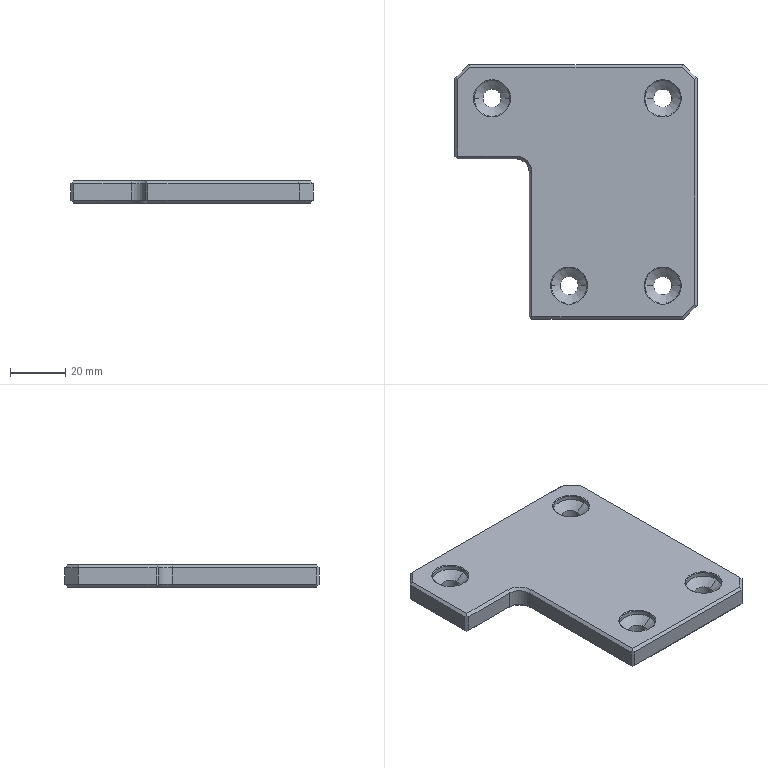Part | Creo | 1 solid | 66 faces | box 88 x 92.5 x 8 mm | volume 49681 mm3 | plane 31 | cone 18 | cylinder 17 | commonest cylinder face diameters 6.6 x8 13 x8 10 x1